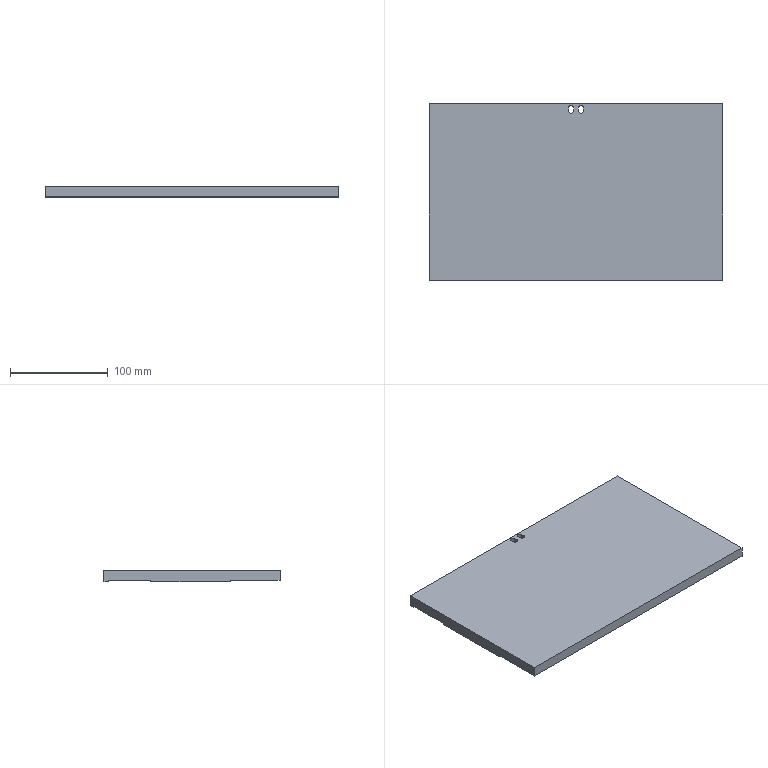Part | SolidWorks | features ICE 3, Extrusion 1, MirrorPattern 1 | 1 solid | 24 faces | box 300 x 180 x 12 mm | volume 604823 mm3 | plane 20 | cylinder 4 | commonest cylinder face diameters 5 x4
STEP:
#1=CARTESIAN_POINT('',(150.,-90.,12.));
#2=VERTEX_POINT('',#1);
#3=CARTESIAN_POINT('',(150.,90.,12.));
#4=VERTEX_POINT('',#3);
#5=CARTESIAN_POINT('',(150.,-90.,12.));
#6=DIRECTION('',(0.,1.,0.));
#7=VECTOR('',#6,1000.);
#8=LINE('',#5,#7);
#9=EDGE_CURVE('',#2,#4,#8,.T.);
#10=ORIENTED_EDGE('',*,*,#9,.T.);
#11=CARTESIAN_POINT('',(-150.,90.,12.));
#12=VERTEX_POINT('',#11);
#13=CARTESIAN_POINT('',(-150.,90.,12.));
#14=DIRECTION('',(-1.,0.,0.));
#15=VECTOR('',#14,1000.);
#16=LINE('',#13,#15);
#17=EDGE_CURVE('',#4,#12,#16,.T.);
#18=ORIENTED_EDGE('',*,*,#17,.T.);
#19=CARTESIAN_POINT('',(-150.,-90.,12.));
#20=VERTEX_POINT('',#19);
#21=CARTESIAN_POINT('',(-150.,-90.,12.));
#22=DIRECTION('',(0.,-1.,0.));
#23=VECTOR('',#22,1000.);
#24=LINE('',#21,#23);
#25=EDGE_CURVE('',#12,#20,#24,.T.);
#26=ORIENTED_EDGE('',*,*,#25,.T.);
#27=CARTESIAN_POINT('',(-150.,-90.,12.));
#28=DIRECTION('',(1.,0.,0.));
#29=VECTOR('',#28,1000.);
#30=LINE('',#27,#29);
#31=EDGE_CURVE('',#20,#2,#30,.T.);
#32=ORIENTED_EDGE('',*,*,#31,.T.);
#33=EDGE_LOOP('',(#10,#18,#26,#32));
#34=FACE_OUTER_BOUND('',#33,.T.);
#35=CARTESIAN_POINT('',(7.5,83.,12.));
#36=VERTEX_POINT('',#35);
#37=CARTESIAN_POINT('',(7.5,86.,12.));
#38=VERTEX_POINT('',#37);
#39=CARTESIAN_POINT('',(7.5,83.,12.));
#40=DIRECTION('',(0.,1.,0.));
#41=VECTOR('',#40,1000.);
#42=LINE('',#39,#41);
#43=EDGE_CURVE('',#36,#38,#42,.T.);
#44=ORIENTED_EDGE('',*,*,#43,.F.);
#45=CARTESIAN_POINT('',(2.5,83.,12.));
#46=VERTEX_POINT('',#45);
#47=CARTESIAN_POINT('',(5.,83.,12.));
#48=DIRECTION('',(0.,0.,1.));
#49=DIRECTION('',(-1.,0.,0.));
#50=AXIS2_PLACEMENT_3D('',#47,#48,#49);
#51=CIRCLE('',#50,2.5);
#52=EDGE_CURVE('',#46,#36,#51,.T.);
#53=ORIENTED_EDGE('',*,*,#52,.F.);
#54=CARTESIAN_POINT('',(2.5,86.,12.));
#55=VERTEX_POINT('',#54);
#56=CARTESIAN_POINT('',(2.5,83.,12.));
#57=DIRECTION('',(0.,-1.,0.));
#58=VECTOR('',#57,1000.);
#59=LINE('',#56,#58);
#60=EDGE_CURVE('',#55,#46,#59,.T.);
#61=ORIENTED_EDGE('',*,*,#60,.F.);
#62=CARTESIAN_POINT('',(5.,86.,12.));
#63=DIRECTION('',(0.,0.,1.));
#64=DIRECTION('',(-1.,0.,0.));
#65=AXIS2_PLACEMENT_3D('',#62,#63,#64);
#66=CIRCLE('',#65,2.5);
#67=EDGE_CURVE('',#38,#55,#66,.T.);
#68=ORIENTED_EDGE('',*,*,#67,.F.);
#69=EDGE_LOOP('',(#44,#53,#61,#68));
#70=FACE_BOUND('',#69,.T.);
#71=CARTESIAN_POINT('',(-2.5,83.,12.));
#72=VERTEX_POINT('',#71);
#73=CARTESIAN_POINT('',(-7.5,83.,12.));
#74=VERTEX_POINT('',#73);
#75=CARTESIAN_POINT('',(-5.,83.,12.));
#76=DIRECTION('',(0.,0.,-1.));
#77=DIRECTION('',(-1.,0.,0.));
#78=AXIS2_PLACEMENT_3D('',#75,#76,#77);
#79=CIRCLE('',#78,2.5);
#80=EDGE_CURVE('',#72,#74,#79,.T.);
#81=ORIENTED_EDGE('',*,*,#80,.T.);
#82=CARTESIAN_POINT('',(-7.5,86.,12.));
#83=VERTEX_POINT('',#82);
#84=CARTESIAN_POINT('',(-7.5,83.,12.));
#85=DIRECTION('',(0.,1.,0.));
#86=VECTOR('',#85,1000.);
#87=LINE('',#84,#86);
#88=EDGE_CURVE('',#74,#83,#87,.T.);
#89=ORIENTED_EDGE('',*,*,#88,.T.);
#90=CARTESIAN_POINT('',(-2.5,86.,12.));
#91=VERTEX_POINT('',#90);
#92=CARTESIAN_POINT('',(-5.,86.,12.));
#93=DIRECTION('',(0.,0.,-1.));
#94=DIRECTION('',(-1.,0.,0.));
#95=AXIS2_PLACEMENT_3D('',#92,#93,#94);
#96=CIRCLE('',#95,2.5);
#97=EDGE_CURVE('',#83,#91,#96,.T.);
#98=ORIENTED_EDGE('',*,*,#97,.T.);
#99=CARTESIAN_POINT('',(-2.5,83.,12.));
#100=DIRECTION('',(0.,-1.,0.));
#101=VECTOR('',#100,1000.);
#102=LINE('',#99,#101);
#103=EDGE_CURVE('',#91,#72,#102,.T.);
#104=ORIENTED_EDGE('',*,*,#103,.T.);
#105=EDGE_LOOP('',(#81,#89,#98,#104));
#106=FACE_BOUND('',#105,.T.);
#107=CARTESIAN_POINT('',(0.,0.,12.));
#108=DIRECTION('',(0.,0.,-1.));
#109=DIRECTION('',(-1.,0.,0.));
#110=AXIS2_PLACEMENT_3D('',#107,#108,#109);
#111=PLANE('',#110);
#112=ADVANCED_FACE('',(#34,#70,#106),#111,.F.);
#113=CARTESIAN_POINT('',(150.,85.,1.5));
#114=VERTEX_POINT('',#113);
#115=CARTESIAN_POINT('',(150.,42.,1.5));
#116=VERTEX_POINT('',#115);
#117=CARTESIAN_POINT('',(150.,42.,1.5));
#118=DIRECTION('',(0.,-1.,0.));
#119=VECTOR('',#118,1000.);
#120=LINE('',#117,#119);
#121=EDGE_CURVE('',#114,#116,#120,.T.);
#122=ORIENTED_EDGE('',*,*,#121,.T.);
#123=CARTESIAN_POINT('',(-150.,42.,1.5));
#124=VERTEX_POINT('',#123);
#125=CARTESIAN_POINT('',(150.,42.,1.5));
#126=DIRECTION('',(-1.,0.,0.));
#127=VECTOR('',#126,1000.);
#128=LINE('',#125,#127);
#129=EDGE_CURVE('',#116,#124,#128,.T.);
#130=ORIENTED_EDGE('',*,*,#129,.T.);
#131=CARTESIAN_POINT('',(-150.,85.,1.5));
#132=VERTEX_POINT('',#131);
#133=CARTESIAN_POINT('',(-150.,42.,1.5));
#134=DIRECTION('',(0.,1.,0.));
#135=VECTOR('',#134,1000.);
#136=LINE('',#133,#135);
#137=EDGE_CURVE('',#124,#132,#136,.T.);
#138=ORIENTED_EDGE('',*,*,#137,.T.);
#139=CARTESIAN_POINT('',(-10.,85.,1.5));
#140=VERTEX_POINT('',#139);
#141=CARTESIAN_POINT('',(150.,85.,1.5));
#142=DIRECTION('',(1.,0.,0.));
#143=VECTOR('',#142,1000.);
#144=LINE('',#141,#143);
#145=EDGE_CURVE('',#132,#140,#144,.T.);
#146=ORIENTED_EDGE('',*,*,#145,.T.);
#147=CARTESIAN_POINT('',(-10.,90.,1.5));
#148=VERTEX_POINT('',#147);
#149=CARTESIAN_POINT('',(-10.,85.,1.5));
#150=DIRECTION('',(0.,1.,0.));
#151=VECTOR('',#150,1000.);
#152=LINE('',#149,#151);
#153=EDGE_CURVE('',#140,#148,#152,.T.);
#154=ORIENTED_EDGE('',*,*,#153,.T.);
#155=CARTESIAN_POINT('',(10.,90.,1.5));
#156=VERTEX_POINT('',#155);
#157=CARTESIAN_POINT('',(10.,90.,1.5));
#158=DIRECTION('',(1.,0.,0.));
#159=VECTOR('',#158,1000.);
#160=LINE('',#157,#159);
#161=EDGE_CURVE('',#148,#156,#160,.T.);
#162=ORIENTED_EDGE('',*,*,#161,.T.);
#163=CARTESIAN_POINT('',(10.,85.,1.5));
#164=VERTEX_POINT('',#163);
#165=CARTESIAN_POINT('',(10.,85.,1.5));
#166=DIRECTION('',(0.,-1.,0.));
#167=VECTOR('',#166,1000.);
#168=LINE('',#165,#167);
#169=EDGE_CURVE('',#156,#164,#168,.T.);
#170=ORIENTED_EDGE('',*,*,#169,.T.);
#171=CARTESIAN_POINT('',(150.,85.,1.5));
#172=DIRECTION('',(1.,0.,0.));
#173=VECTOR('',#172,1000.);
#174=LINE('',#171,#173);
#175=EDGE_CURVE('',#164,#114,#174,.T.);
#176=ORIENTED_EDGE('',*,*,#175,.T.);
#177=EDGE_LOOP('',(#122,#130,#138,#146,#154,#162,#170,#176));
#178=FACE_OUTER_BOUND('',#177,.T.);
#179=CARTESIAN_POINT('',(2.5,83.,1.5));
#180=VERTEX_POINT('',#179);
#181=CARTESIAN_POINT('',(2.5,86.,1.5));
#182=VERTEX_POINT('',#181);
#183=CARTESIAN_POINT('',(2.5,83.,1.5));
#184=DIRECTION('',(0.,1.,0.));
#185=VECTOR('',#184,1000.);
#186=LINE('',#183,#185);
#187=EDGE_CURVE('',#180,#182,#186,.T.);
#188=ORIENTED_EDGE('',*,*,#187,.F.);
#189=CARTESIAN_POINT('',(7.5,83.,1.5));
#190=VERTEX_POINT('',#189);
#191=CARTESIAN_POINT('',(5.,83.,1.5));
#192=DIRECTION('',(0.,0.,-1.));
#193=DIRECTION('',(-1.,0.,0.));
#194=AXIS2_PLACEMENT_3D('',#191,#192,#193);
#195=CIRCLE('',#194,2.5);
#196=EDGE_CURVE('',#190,#180,#195,.T.);
#197=ORIENTED_EDGE('',*,*,#196,.F.);
#198=CARTESIAN_POINT('',(7.5,86.,1.5));
#199=VERTEX_POINT('',#198);
#200=CARTESIAN_POINT('',(7.5,83.,1.5));
#201=DIRECTION('',(0.,-1.,0.));
#202=VECTOR('',#201,1000.);
#203=LINE('',#200,#202);
#204=EDGE_CURVE('',#199,#190,#203,.T.);
#205=ORIENTED_EDGE('',*,*,#204,.F.);
#206=CARTESIAN_POINT('',(5.,86.,1.5));
#207=DIRECTION('',(0.,0.,-1.));
#208=DIRECTION('',(-1.,0.,0.));
#209=AXIS2_PLACEMENT_3D('',#206,#207,#208);
#210=CIRCLE('',#209,2.5);
#211=EDGE_CURVE('',#182,#199,#210,.T.);
#212=ORIENTED_EDGE('',*,*,#211,.F.);
#213=EDGE_LOOP('',(#188,#197,#205,#212));
#214=FACE_BOUND('',#213,.T.);
#215=CARTESIAN_POINT('',(-7.5,83.,1.5));
#216=VERTEX_POINT('',#215);
#217=CARTESIAN_POINT('',(-2.5,83.,1.5));
#218=VERTEX_POINT('',#217);
#219=CARTESIAN_POINT('',(-5.,83.,1.5));
#220=DIRECTION('',(0.,0.,1.));
#221=DIRECTION('',(1.,0.,0.));
#222=AXIS2_PLACEMENT_3D('',#219,#220,#221);
#223=CIRCLE('',#222,2.5);
#224=EDGE_CURVE('',#216,#218,#223,.T.);
#225=ORIENTED_EDGE('',*,*,#224,.T.);
#226=CARTESIAN_POINT('',(-2.5,86.,1.5));
#227=VERTEX_POINT('',#226);
#228=CARTESIAN_POINT('',(-2.5,83.,1.5));
#229=DIRECTION('',(0.,1.,0.));
#230=VECTOR('',#229,1000.);
#231=LINE('',#228,#230);
#232=EDGE_CURVE('',#218,#227,#231,.T.);
#233=ORIENTED_EDGE('',*,*,#232,.T.);
#234=CARTESIAN_POINT('',(-7.5,86.,1.5));
#235=VERTEX_POINT('',#234);
#236=CARTESIAN_POINT('',(-5.,86.,1.5));
#237=DIRECTION('',(0.,0.,1.));
#238=DIRECTION('',(1.,0.,0.));
#239=AXIS2_PLACEMENT_3D('',#236,#237,#238);
#240=CIRCLE('',#239,2.5);
#241=EDGE_CURVE('',#227,#235,#240,.T.);
#242=ORIENTED_EDGE('',*,*,#241,.T.);
#243=CARTESIAN_POINT('',(-7.5,83.,1.5));
#244=DIRECTION('',(0.,-1.,0.));
#245=VECTOR('',#244,1000.);
#246=LINE('',#243,#245);
#247=EDGE_CURVE('',#235,#216,#246,.T.);
#248=ORIENTED_EDGE('',*,*,#247,.T.);
#249=EDGE_LOOP('',(#225,#233,#242,#248));
#250=FACE_BOUND('',#249,.T.);
#251=CARTESIAN_POINT('',(0.,0.,1.5));
#252=DIRECTION('',(0.,0.,1.));
#253=DIRECTION('',(1.,0.,0.));
#254=AXIS2_PLACEMENT_3D('',#251,#252,#253);
#255=PLANE('',#254);
#256=ADVANCED_FACE('',(#178,#214,#250),#255,.F.);
#257=CARTESIAN_POINT('',(10.,90.,0.));
#258=VERTEX_POINT('',#257);
#259=CARTESIAN_POINT('',(10.,85.,0.));
#260=VERTEX_POINT('',#259);
#261=CARTESIAN_POINT('',(10.,85.,0.));
#262=DIRECTION('',(0.,-1.,0.));
#263=VECTOR('',#262,1000.);
#264=LINE('',#261,#263);
#265=EDGE_CURVE('',#258,#260,#264,.T.);
#266=ORIENTED_EDGE('',*,*,#265,.F.);
#267=CARTESIAN_POINT('',(150.,90.,0.));
#268=VERTEX_POINT('',#267);
#269=CARTESIAN_POINT('',(-150.,90.,0.));
#270=DIRECTION('',(-1.,0.,0.));
#271=VECTOR('',#270,1000.);
#272=LINE('',#269,#271);
#273=EDGE_CURVE('',#268,#258,#272,.T.);
#274=ORIENTED_EDGE('',*,*,#273,.F.);
#275=CARTESIAN_POINT('',(150.,85.,0.));
#276=VERTEX_POINT('',#275);
#277=CARTESIAN_POINT('',(150.,-90.,0.));
#278=DIRECTION('',(0.,1.,0.));
#279=VECTOR('',#278,1000.);
#280=LINE('',#277,#279);
#281=EDGE_CURVE('',#276,#268,#280,.T.);
#282=ORIENTED_EDGE('',*,*,#281,.F.);
#283=CARTESIAN_POINT('',(150.,85.,0.));
#284=DIRECTION('',(1.,0.,0.));
#285=VECTOR('',#284,1000.);
#286=LINE('',#283,#285);
#287=EDGE_CURVE('',#260,#276,#286,.T.);
#288=ORIENTED_EDGE('',*,*,#287,.F.);
#289=EDGE_LOOP('',(#266,#274,#282,#288));
#290=FACE_OUTER_BOUND('',#289,.T.);
#291=CARTESIAN_POINT('',(0.,0.,0.));
#292=DIRECTION('',(0.,0.,-1.));
#293=DIRECTION('',(-1.,0.,0.));
#294=AXIS2_PLACEMENT_3D('',#291,#292,#293);
#295=PLANE('',#294);
#296=ADVANCED_FACE('',(#290),#295,.T.);
#297=ORIENTED_EDGE('',*,*,#175,.F.);
#298=CARTESIAN_POINT('',(10.,85.,22.116));
#299=DIRECTION('',(0.,0.,-1.));
#300=VECTOR('',#299,1000.);
#301=LINE('',#298,#300);
#302=EDGE_CURVE('',#164,#260,#301,.T.);
#303=ORIENTED_EDGE('',*,*,#302,.T.);
#304=ORIENTED_EDGE('',*,*,#287,.T.);
#305=CARTESIAN_POINT('',(150.,85.,1.5));
#306=DIRECTION('',(0.,0.,-1.));
#307=VECTOR('',#306,1000.);
#308=LINE('',#305,#307);
#309=EDGE_CURVE('',#114,#276,#308,.T.);
#310=ORIENTED_EDGE('',*,*,#309,.F.);
#311=EDGE_LOOP('',(#297,#303,#304,#310));
#312=FACE_OUTER_BOUND('',#311,.T.);
#313=CARTESIAN_POINT('',(150.,85.,1.5));
#314=DIRECTION('',(0.,1.,0.));
#315=DIRECTION('',(0.,0.,1.));
#316=AXIS2_PLACEMENT_3D('',#313,#314,#315);
#317=PLANE('',#316);
#318=ADVANCED_FACE('',(#312),#317,.F.);
#319=CARTESIAN_POINT('',(-10.,85.,0.));
#320=VERTEX_POINT('',#319);
#321=CARTESIAN_POINT('',(-10.,90.,0.));
#322=VERTEX_POINT('',#321);
#323=CARTESIAN_POINT('',(-10.,85.,0.));
#324=DIRECTION('',(0.,1.,0.));
#325=VECTOR('',#324,1000.);
#326=LINE('',#323,#325);
#327=EDGE_CURVE('',#320,#322,#326,.T.);
#328=ORIENTED_EDGE('',*,*,#327,.F.);
#329=CARTESIAN_POINT('',(-150.,85.,0.));
#330=VERTEX_POINT('',#329);
#331=CARTESIAN_POINT('',(150.,85.,0.));
#332=DIRECTION('',(1.,0.,0.));
#333=VECTOR('',#332,1000.);
#334=LINE('',#331,#333);
#335=EDGE_CURVE('',#330,#320,#334,.T.);
#336=ORIENTED_EDGE('',*,*,#335,.F.);
#337=CARTESIAN_POINT('',(-150.,90.,0.));
#338=VERTEX_POINT('',#337);
#339=CARTESIAN_POINT('',(-150.,-90.,0.));
#340=DIRECTION('',(0.,-1.,0.));
#341=VECTOR('',#340,1000.);
#342=LINE('',#339,#341);
#343=EDGE_CURVE('',#338,#330,#342,.T.);
#344=ORIENTED_EDGE('',*,*,#343,.F.);
#345=CARTESIAN_POINT('',(-150.,90.,0.));
#346=DIRECTION('',(-1.,0.,0.));
#347=VECTOR('',#346,1000.);
#348=LINE('',#345,#347);
#349=EDGE_CURVE('',#322,#338,#348,.T.);
#350=ORIENTED_EDGE('',*,*,#349,.F.);
#351=EDGE_LOOP('',(#328,#336,#344,#350));
#352=FACE_OUTER_BOUND('',#351,.T.);
#353=CARTESIAN_POINT('',(0.,0.,0.));
#354=DIRECTION('',(0.,0.,-1.));
#355=DIRECTION('',(-1.,0.,0.));
#356=AXIS2_PLACEMENT_3D('',#353,#354,#355);
#357=PLANE('',#356);
#358=ADVANCED_FACE('',(#352),#357,.T.);
#359=ORIENTED_EDGE('',*,*,#121,.F.);
#360=ORIENTED_EDGE('',*,*,#309,.T.);
#361=ORIENTED_EDGE('',*,*,#281,.T.);
#362=CARTESIAN_POINT('',(150.,90.,12.));
#363=DIRECTION('',(0.,0.,-1.));
#364=VECTOR('',#363,1000.);
#365=LINE('',#362,#364);
#366=EDGE_CURVE('',#4,#268,#365,.T.);
#367=ORIENTED_EDGE('',*,*,#366,.F.);
#368=ORIENTED_EDGE('',*,*,#9,.F.);
#369=CARTESIAN_POINT('',(150.,-90.,1.5));
#370=VERTEX_POINT('',#369);
#371=CARTESIAN_POINT('',(150.,-90.,12.));
#372=DIRECTION('',(0.,0.,-1.));
#373=VECTOR('',#372,1000.);
#374=LINE('',#371,#373);
#375=EDGE_CURVE('',#2,#370,#374,.T.);
#376=ORIENTED_EDGE('',*,*,#375,.T.);
#377=CARTESIAN_POINT('',(150.,-39.,1.5));
#378=VERTEX_POINT('',#377);
#379=CARTESIAN_POINT('',(150.,-90.,1.5));
#380=DIRECTION('',(0.,-1.,0.));
#381=VECTOR('',#380,1000.);
#382=LINE('',#379,#381);
#383=EDGE_CURVE('',#378,#370,#382,.T.);
#384=ORIENTED_EDGE('',*,*,#383,.F.);
#385=CARTESIAN_POINT('',(150.,-39.,0.));
#386=VERTEX_POINT('',#385);
#387=CARTESIAN_POINT('',(150.,-39.,1.5));
#388=DIRECTION('',(0.,0.,-1.));
#389=VECTOR('',#388,1000.);
#390=LINE('',#387,#389);
#391=EDGE_CURVE('',#378,#386,#390,.T.);
#392=ORIENTED_EDGE('',*,*,#391,.T.);
#393=CARTESIAN_POINT('',(150.,42.,0.));
#394=VERTEX_POINT('',#393);
#395=CARTESIAN_POINT('',(150.,-90.,0.));
#396=DIRECTION('',(0.,1.,0.));
#397=VECTOR('',#396,1000.);
#398=LINE('',#395,#397);
#399=EDGE_CURVE('',#386,#394,#398,.T.);
#400=ORIENTED_EDGE('',*,*,#399,.T.);
#401=CARTESIAN_POINT('',(150.,42.,1.5));
#402=DIRECTION('',(0.,0.,-1.));
#403=VECTOR('',#402,1000.);
#404=LINE('',#401,#403);
#405=EDGE_CURVE('',#116,#394,#404,.T.);
#406=ORIENTED_EDGE('',*,*,#405,.F.);
#407=EDGE_LOOP('',(#359,#360,#361,#367,#368,#376,#384,#392,#400,#406));
#408=FACE_OUTER_BOUND('',#407,.T.);
#409=CARTESIAN_POINT('',(150.,-90.,12.));
#410=DIRECTION('',(-1.,0.,0.));
#411=DIRECTION('',(0.,0.,1.));
#412=AXIS2_PLACEMENT_3D('',#409,#410,#411);
#413=PLANE('',#412);
#414=ADVANCED_FACE('',(#408),#413,.F.);
#415=ORIENTED_EDGE('',*,*,#273,.T.);
#416=CARTESIAN_POINT('',(10.,90.,22.116));
#417=DIRECTION('',(0.,0.,-1.));
#418=VECTOR('',#417,1000.);
#419=LINE('',#416,#418);
#420=EDGE_CURVE('',#156,#258,#419,.T.);
#421=ORIENTED_EDGE('',*,*,#420,.F.);
#422=ORIENTED_EDGE('',*,*,#161,.F.);
#423=CARTESIAN_POINT('',(-10.,90.,22.116));
#424=DIRECTION('',(0.,0.,-1.));
#425=VECTOR('',#424,1000.);
#426=LINE('',#423,#425);
#427=EDGE_CURVE('',#148,#322,#426,.T.);
#428=ORIENTED_EDGE('',*,*,#427,.T.);
#429=ORIENTED_EDGE('',*,*,#349,.T.);
#430=CARTESIAN_POINT('',(-150.,90.,12.));
#431=DIRECTION('',(0.,0.,-1.));
#432=VECTOR('',#431,1000.);
#433=LINE('',#430,#432);
#434=EDGE_CURVE('',#12,#338,#433,.T.);
#435=ORIENTED_EDGE('',*,*,#434,.F.);
#436=ORIENTED_EDGE('',*,*,#17,.F.);
#437=ORIENTED_EDGE('',*,*,#366,.T.);
#438=EDGE_LOOP('',(#415,#421,#422,#428,#429,#435,#436,#437));
#439=FACE_OUTER_BOUND('',#438,.T.);
#440=CARTESIAN_POINT('',(-150.,90.,12.));
#441=DIRECTION('',(0.,-1.,0.));
#442=DIRECTION('',(0.,0.,-1.));
#443=AXIS2_PLACEMENT_3D('',#440,#441,#442);
#444=PLANE('',#443);
#445=ADVANCED_FACE('',(#439),#444,.F.);
#446=ORIENTED_EDGE('',*,*,#343,.T.);
#447=CARTESIAN_POINT('',(-150.,85.,1.5));
#448=DIRECTION('',(0.,0.,-1.));
#449=VECTOR('',#448,1000.);
#450=LINE('',#447,#449);
#451=EDGE_CURVE('',#132,#330,#450,.T.);
#452=ORIENTED_EDGE('',*,*,#451,.F.);
#453=ORIENTED_EDGE('',*,*,#137,.F.);
#454=CARTESIAN_POINT('',(-150.,42.,0.));
#455=VERTEX_POINT('',#454);
#456=CARTESIAN_POINT('',(-150.,42.,1.5));
#457=DIRECTION('',(0.,0.,-1.));
#458=VECTOR('',#457,1000.);
#459=LINE('',#456,#458);
#460=EDGE_CURVE('',#124,#455,#459,.T.);
#461=ORIENTED_EDGE('',*,*,#460,.T.);
#462=CARTESIAN_POINT('',(-150.,-39.,0.));
#463=VERTEX_POINT('',#462);
#464=CARTESIAN_POINT('',(-150.,-90.,0.));
#465=DIRECTION('',(0.,-1.,0.));
#466=VECTOR('',#465,1000.);
#467=LINE('',#464,#466);
#468=EDGE_CURVE('',#455,#463,#467,.T.);
#469=ORIENTED_EDGE('',*,*,#468,.T.);
#470=CARTESIAN_POINT('',(-150.,-39.,1.5));
#471=VERTEX_POINT('',#470);
#472=CARTESIAN_POINT('',(-150.,-39.,1.5));
#473=DIRECTION('',(0.,0.,-1.));
#474=VECTOR('',#473,1000.);
#475=LINE('',#472,#474);
#476=EDGE_CURVE('',#471,#463,#475,.T.);
#477=ORIENTED_EDGE('',*,*,#476,.F.);
#478=CARTESIAN_POINT('',(-150.,-90.,1.5));
#479=VERTEX_POINT('',#478);
#480=CARTESIAN_POINT('',(-150.,-90.,1.5));
#481=DIRECTION('',(0.,1.,0.));
#482=VECTOR('',#481,1000.);
#483=LINE('',#480,#482);
#484=EDGE_CURVE('',#479,#471,#483,.T.);
#485=ORIENTED_EDGE('',*,*,#484,.F.);
#486=CARTESIAN_POINT('',(-150.,-90.,12.));
#487=DIRECTION('',(0.,0.,-1.));
#488=VECTOR('',#487,1000.);
#489=LINE('',#486,#488);
#490=EDGE_CURVE('',#20,#479,#489,.T.);
#491=ORIENTED_EDGE('',*,*,#490,.F.);
#492=ORIENTED_EDGE('',*,*,#25,.F.);
#493=ORIENTED_EDGE('',*,*,#434,.T.);
#494=EDGE_LOOP('',(#446,#452,#453,#461,#469,#477,#485,#491,#492,#493));
#495=FACE_OUTER_BOUND('',#494,.T.);
#496=CARTESIAN_POINT('',(-150.,-90.,12.));
#497=DIRECTION('',(1.,0.,0.));
#498=DIRECTION('',(0.,0.,-1.));
#499=AXIS2_PLACEMENT_3D('',#496,#497,#498);
#500=PLANE('',#499);
#501=ADVANCED_FACE('',(#495),#500,.F.);
#502=ORIENTED_EDGE('',*,*,#490,.T.);
#503=CARTESIAN_POINT('',(150.,-90.,1.5));
#504=DIRECTION('',(-1.,0.,0.));
#505=VECTOR('',#504,1000.);
#506=LINE('',#503,#505);
#507=EDGE_CURVE('',#370,#479,#506,.T.);
#508=ORIENTED_EDGE('',*,*,#507,.F.);
#509=ORIENTED_EDGE('',*,*,#375,.F.);
#510=ORIENTED_EDGE('',*,*,#31,.F.);
#511=EDGE_LOOP('',(#502,#508,#509,#510));
#512=FACE_OUTER_BOUND('',#511,.T.);
#513=CARTESIAN_POINT('',(-150.,-90.,12.));
#514=DIRECTION('',(0.,1.,0.));
#515=DIRECTION('',(0.,0.,1.));
#516=AXIS2_PLACEMENT_3D('',#513,#514,#515);
#517=PLANE('',#516);
#518=ADVANCED_FACE('',(#512),#517,.F.);
#519=CARTESIAN_POINT('',(150.,42.,0.));
#520=DIRECTION('',(-1.,0.,0.));
#521=VECTOR('',#520,1000.);
#522=LINE('',#519,#521);
#523=EDGE_CURVE('',#394,#455,#522,.T.);
#524=ORIENTED_EDGE('',*,*,#523,.F.);
#525=ORIENTED_EDGE('',*,*,#399,.F.);
#526=CARTESIAN_POINT('',(150.,-39.,0.));
#527=DIRECTION('',(1.,0.,0.));
#528=VECTOR('',#527,1000.);
#529=LINE('',#526,#528);
#530=EDGE_CURVE('',#463,#386,#529,.T.);
#531=ORIENTED_EDGE('',*,*,#530,.F.);
#532=ORIENTED_EDGE('',*,*,#468,.F.);
#533=EDGE_LOOP('',(#524,#525,#531,#532));
#534=FACE_OUTER_BOUND('',#533,.T.);
#535=CARTESIAN_POINT('',(0.,0.,0.));
#536=DIRECTION('',(0.,0.,-1.));
#537=DIRECTION('',(-1.,0.,0.));
#538=AXIS2_PLACEMENT_3D('',#535,#536,#537);
#539=PLANE('',#538);
#540=ADVANCED_FACE('',(#534),#539,.T.);
#541=ORIENTED_EDGE('',*,*,#530,.T.);
#542=ORIENTED_EDGE('',*,*,#391,.F.);
#543=CARTESIAN_POINT('',(150.,-39.,1.5));
#544=DIRECTION('',(1.,0.,0.));
#545=VECTOR('',#544,1000.);
#546=LINE('',#543,#545);
#547=EDGE_CURVE('',#471,#378,#546,.T.);
#548=ORIENTED_EDGE('',*,*,#547,.F.);
#549=ORIENTED_EDGE('',*,*,#476,.T.);
#550=EDGE_LOOP('',(#541,#542,#548,#549));
#551=FACE_OUTER_BOUND('',#550,.T.);
#552=CARTESIAN_POINT('',(150.,-39.,1.5));
#553=DIRECTION('',(0.,1.,0.));
#554=DIRECTION('',(0.,0.,1.));
#555=AXIS2_PLACEMENT_3D('',#552,#553,#554);
#556=PLANE('',#555);
#557=ADVANCED_FACE('',(#551),#556,.F.);
#558=ORIENTED_EDGE('',*,*,#383,.T.);
#559=ORIENTED_EDGE('',*,*,#507,.T.);
#560=ORIENTED_EDGE('',*,*,#484,.T.);
#561=ORIENTED_EDGE('',*,*,#547,.T.);
#562=EDGE_LOOP('',(#558,#559,#560,#561));
#563=FACE_OUTER_BOUND('',#562,.T.);
#564=CARTESIAN_POINT('',(0.,0.,1.5));
#565=DIRECTION('',(0.,0.,1.));
#566=DIRECTION('',(1.,0.,0.));
#567=AXIS2_PLACEMENT_3D('',#564,#565,#566);
#568=PLANE('',#567);
#569=ADVANCED_FACE('',(#563),#568,.F.);
#570=ORIENTED_EDGE('',*,*,#335,.T.);
#571=CARTESIAN_POINT('',(-10.,85.,22.116));
#572=DIRECTION('',(0.,0.,-1.));
#573=VECTOR('',#572,1000.);
#574=LINE('',#571,#573);
#575=EDGE_CURVE('',#140,#320,#574,.T.);
#576=ORIENTED_EDGE('',*,*,#575,.F.);
#577=ORIENTED_EDGE('',*,*,#145,.F.);
#578=ORIENTED_EDGE('',*,*,#451,.T.);
#579=EDGE_LOOP('',(#570,#576,#577,#578));
#580=FACE_OUTER_BOUND('',#579,.T.);
#581=CARTESIAN_POINT('',(150.,85.,1.5));
#582=DIRECTION('',(0.,1.,0.));
#583=DIRECTION('',(0.,0.,1.));
#584=AXIS2_PLACEMENT_3D('',#581,#582,#583);
#585=PLANE('',#584);
#586=ADVANCED_FACE('',(#580),#585,.F.);
#587=ORIENTED_EDGE('',*,*,#523,.T.);
#588=ORIENTED_EDGE('',*,*,#460,.F.);
#589=ORIENTED_EDGE('',*,*,#129,.F.);
#590=ORIENTED_EDGE('',*,*,#405,.T.);
#591=EDGE_LOOP('',(#587,#588,#589,#590));
#592=FACE_OUTER_BOUND('',#591,.T.);
#593=CARTESIAN_POINT('',(150.,42.,1.5));
#594=DIRECTION('',(0.,-1.,0.));
#595=DIRECTION('',(0.,0.,-1.));
#596=AXIS2_PLACEMENT_3D('',#593,#594,#595);
#597=PLANE('',#596);
#598=ADVANCED_FACE('',(#592),#597,.F.);
#599=ORIENTED_EDGE('',*,*,#420,.T.);
#600=ORIENTED_EDGE('',*,*,#265,.T.);
#601=ORIENTED_EDGE('',*,*,#302,.F.);
#602=ORIENTED_EDGE('',*,*,#169,.F.);
#603=EDGE_LOOP('',(#599,#600,#601,#602));
#604=FACE_OUTER_BOUND('',#603,.T.);
#605=CARTESIAN_POINT('',(10.,85.,22.116));
#606=DIRECTION('',(1.,0.,0.));
#607=DIRECTION('',(0.,0.,-1.));
#608=AXIS2_PLACEMENT_3D('',#605,#606,#607);
#609=PLANE('',#608);
#610=ADVANCED_FACE('',(#604),#609,.F.);
#611=ORIENTED_EDGE('',*,*,#575,.T.);
#612=ORIENTED_EDGE('',*,*,#327,.T.);
#613=ORIENTED_EDGE('',*,*,#427,.F.);
#614=ORIENTED_EDGE('',*,*,#153,.F.);
#615=EDGE_LOOP('',(#611,#612,#613,#614));
#616=FACE_OUTER_BOUND('',#615,.T.);
#617=CARTESIAN_POINT('',(-10.,85.,22.116));
#618=DIRECTION('',(-1.,0.,0.));
#619=DIRECTION('',(0.,0.,1.));
#620=AXIS2_PLACEMENT_3D('',#617,#618,#619);
#621=PLANE('',#620);
#622=ADVANCED_FACE('',(#616),#621,.F.);
#623=ORIENTED_EDGE('',*,*,#52,.T.);
#624=CARTESIAN_POINT('',(7.5,83.,12.001));
#625=DIRECTION('',(0.,0.,-1.));
#626=VECTOR('',#625,1000.);
#627=LINE('',#624,#626);
#628=EDGE_CURVE('',#36,#190,#627,.T.);
#629=ORIENTED_EDGE('',*,*,#628,.T.);
#630=ORIENTED_EDGE('',*,*,#196,.T.);
#631=CARTESIAN_POINT('',(2.5,83.,12.001));
#632=DIRECTION('',(0.,0.,-1.));
#633=VECTOR('',#632,1000.);
#634=LINE('',#631,#633);
#635=EDGE_CURVE('',#46,#180,#634,.T.);
#636=ORIENTED_EDGE('',*,*,#635,.F.);
#637=EDGE_LOOP('',(#623,#629,#630,#636));
#638=FACE_OUTER_BOUND('',#637,.T.);
#639=CARTESIAN_POINT('',(5.,83.,12.001));
#640=DIRECTION('',(0.,0.,-1.));
#641=DIRECTION('',(-1.,0.,0.));
#642=AXIS2_PLACEMENT_3D('',#639,#640,#641);
#643=CYLINDRICAL_SURFACE('',#642,2.5);
#644=ADVANCED_FACE('',(#638),#643,.F.);
#645=ORIENTED_EDGE('',*,*,#43,.T.);
#646=CARTESIAN_POINT('',(7.5,86.,12.001));
#647=DIRECTION('',(0.,0.,-1.));
#648=VECTOR('',#647,1000.);
#649=LINE('',#646,#648);
#650=EDGE_CURVE('',#38,#199,#649,.T.);
#651=ORIENTED_EDGE('',*,*,#650,.T.);
#652=ORIENTED_EDGE('',*,*,#204,.T.);
#653=ORIENTED_EDGE('',*,*,#628,.F.);
#654=EDGE_LOOP('',(#645,#651,#652,#653));
#655=FACE_OUTER_BOUND('',#654,.T.);
#656=CARTESIAN_POINT('',(7.5,83.,12.001));
#657=DIRECTION('',(1.,0.,0.));
#658=DIRECTION('',(0.,0.,-1.));
#659=AXIS2_PLACEMENT_3D('',#656,#657,#658);
#660=PLANE('',#659);
#661=ADVANCED_FACE('',(#655),#660,.F.);
#662=ORIENTED_EDGE('',*,*,#67,.T.);
#663=CARTESIAN_POINT('',(2.5,86.,12.001));
#664=DIRECTION('',(0.,0.,-1.));
#665=VECTOR('',#664,1000.);
#666=LINE('',#663,#665);
#667=EDGE_CURVE('',#55,#182,#666,.T.);
#668=ORIENTED_EDGE('',*,*,#667,.T.);
#669=ORIENTED_EDGE('',*,*,#211,.T.);
#670=ORIENTED_EDGE('',*,*,#650,.F.);
#671=EDGE_LOOP('',(#662,#668,#669,#670));
#672=FACE_OUTER_BOUND('',#671,.T.);
#673=CARTESIAN_POINT('',(5.,86.,12.001));
#674=DIRECTION('',(0.,0.,-1.));
#675=DIRECTION('',(-1.,0.,0.));
#676=AXIS2_PLACEMENT_3D('',#673,#674,#675);
#677=CYLINDRICAL_SURFACE('',#676,2.5);
#678=ADVANCED_FACE('',(#672),#677,.F.);
#679=ORIENTED_EDGE('',*,*,#60,.T.);
#680=ORIENTED_EDGE('',*,*,#635,.T.);
#681=ORIENTED_EDGE('',*,*,#187,.T.);
#682=ORIENTED_EDGE('',*,*,#667,.F.);
#683=EDGE_LOOP('',(#679,#680,#681,#682));
#684=FACE_OUTER_BOUND('',#683,.T.);
#685=CARTESIAN_POINT('',(2.5,83.,12.001));
#686=DIRECTION('',(-1.,0.,0.));
#687=DIRECTION('',(0.,0.,1.));
#688=AXIS2_PLACEMENT_3D('',#685,#686,#687);
#689=PLANE('',#688);
#690=ADVANCED_FACE('',(#684),#689,.F.);
#691=CARTESIAN_POINT('',(-2.5,83.,12.001));
#692=DIRECTION('',(0.,0.,-1.));
#693=VECTOR('',#692,1000.);
#694=LINE('',#691,#693);
#695=EDGE_CURVE('',#72,#218,#694,.T.);
#696=ORIENTED_EDGE('',*,*,#695,.T.);
#697=ORIENTED_EDGE('',*,*,#224,.F.);
#698=CARTESIAN_POINT('',(-7.5,83.,12.001));
#699=DIRECTION('',(0.,0.,-1.));
#700=VECTOR('',#699,1000.);
#701=LINE('',#698,#700);
#702=EDGE_CURVE('',#74,#216,#701,.T.);
#703=ORIENTED_EDGE('',*,*,#702,.F.);
#704=ORIENTED_EDGE('',*,*,#80,.F.);
#705=EDGE_LOOP('',(#696,#697,#703,#704));
#706=FACE_OUTER_BOUND('',#705,.T.);
#707=CARTESIAN_POINT('',(-5.,83.,12.001));
#708=DIRECTION('',(0.,0.,-1.));
#709=DIRECTION('',(-1.,0.,0.));
#710=AXIS2_PLACEMENT_3D('',#707,#708,#709);
#711=CYLINDRICAL_SURFACE('',#710,2.5);
#712=ADVANCED_FACE('',(#706),#711,.F.);
#713=CARTESIAN_POINT('',(-2.5,86.,12.001));
#714=DIRECTION('',(0.,0.,-1.));
#715=VECTOR('',#714,1000.);
#716=LINE('',#713,#715);
#717=EDGE_CURVE('',#91,#227,#716,.T.);
#718=ORIENTED_EDGE('',*,*,#717,.T.);
#719=ORIENTED_EDGE('',*,*,#232,.F.);
#720=ORIENTED_EDGE('',*,*,#695,.F.);
#721=ORIENTED_EDGE('',*,*,#103,.F.);
#722=EDGE_LOOP('',(#718,#719,#720,#721));
#723=FACE_OUTER_BOUND('',#722,.T.);
#724=CARTESIAN_POINT('',(-2.5,83.,12.001));
#725=DIRECTION('',(-1.,0.,0.));
#726=DIRECTION('',(0.,0.,1.));
#727=AXIS2_PLACEMENT_3D('',#724,#725,#726);
#728=PLANE('',#727);
#729=ADVANCED_FACE('',(#723),#728,.T.);
#730=CARTESIAN_POINT('',(-7.5,86.,12.001));
#731=DIRECTION('',(0.,0.,-1.));
#732=VECTOR('',#731,1000.);
#733=LINE('',#730,#732);
#734=EDGE_CURVE('',#83,#235,#733,.T.);
#735=ORIENTED_EDGE('',*,*,#734,.T.);
#736=ORIENTED_EDGE('',*,*,#241,.F.);
#737=ORIENTED_EDGE('',*,*,#717,.F.);
#738=ORIENTED_EDGE('',*,*,#97,.F.);
#739=EDGE_LOOP('',(#735,#736,#737,#738));
#740=FACE_OUTER_BOUND('',#739,.T.);
#741=CARTESIAN_POINT('',(-5.,86.,12.001));
#742=DIRECTION('',(0.,0.,-1.));
#743=DIRECTION('',(-1.,0.,0.));
#744=AXIS2_PLACEMENT_3D('',#741,#742,#743);
#745=CYLINDRICAL_SURFACE('',#744,2.5);
#746=ADVANCED_FACE('',(#740),#745,.F.);
#747=ORIENTED_EDGE('',*,*,#702,.T.);
#748=ORIENTED_EDGE('',*,*,#247,.F.);
#749=ORIENTED_EDGE('',*,*,#734,.F.);
#750=ORIENTED_EDGE('',*,*,#88,.F.);
#751=EDGE_LOOP('',(#747,#748,#749,#750));
#752=FACE_OUTER_BOUND('',#751,.T.);
#753=CARTESIAN_POINT('',(-7.5,83.,12.001));
#754=DIRECTION('',(1.,0.,0.));
#755=DIRECTION('',(0.,0.,-1.));
#756=AXIS2_PLACEMENT_3D('',#753,#754,#755);
#757=PLANE('',#756);
#758=ADVANCED_FACE('',(#752),#757,.T.);
#759=CLOSED_SHELL('',(#112,#256,#296,#318,#358,#414,#445,#501,#518,#540,#557,#569,#586,#598,#610,#622,#644,#661,#678,#690,#712,#729,#746,#758));
#760=MANIFOLD_SOLID_BREP('',#759);
#761=CARTESIAN_POINT('',(0.,0.,0.));
#762=DIRECTION('',(0.,0.,1.));
#763=DIRECTION('',(1.,0.,0.));
#764=AXIS2_PLACEMENT_3D('',#761,#762,#763);
#765=(LENGTH_UNIT()NAMED_UNIT(*)SI_UNIT(.MILLI.,.METRE.));
#766=UNCERTAINTY_MEASURE_WITH_UNIT(LENGTH_MEASURE(0.00001),#765,'','');
#767=(NAMED_UNIT(*)PLANE_ANGLE_UNIT()SI_UNIT($,.RADIAN.));
#768=(NAMED_UNIT(*)SI_UNIT($,.STERADIAN.)SOLID_ANGLE_UNIT());
#769=(GEOMETRIC_REPRESENTATION_CONTEXT(3)GLOBAL_UNCERTAINTY_ASSIGNED_CONTEXT((#766))GLOBAL_UNIT_ASSIGNED_CONTEXT((#765,#767,#768))REPRESENTATION_CONTEXT('',''));
#770=ADVANCED_BREP_SHAPE_REPRESENTATION('',(#760,#764),#769);